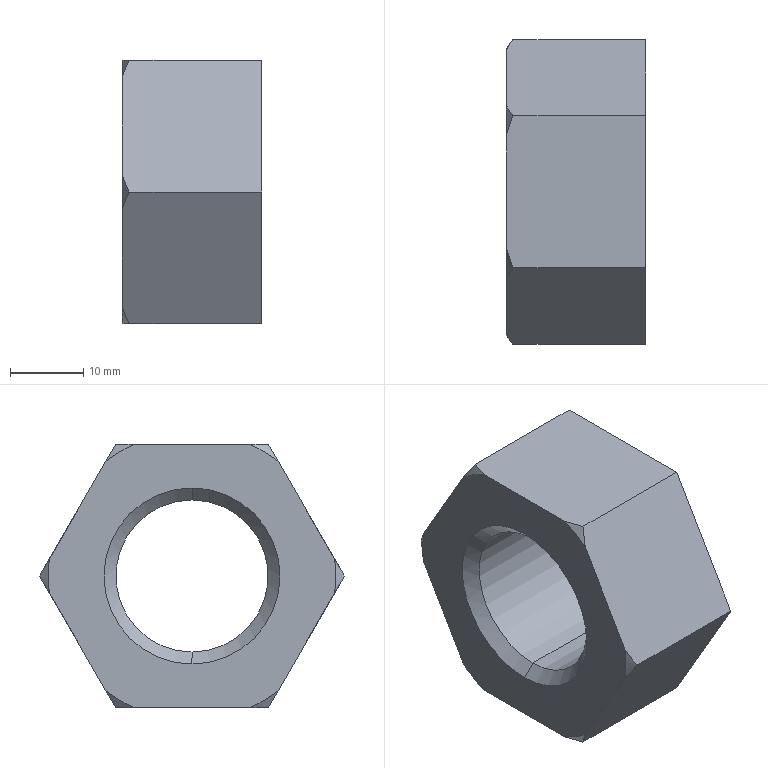Part | STEP file | 11-FJFN24nut11 | 1 solid | 20 faces | box 19 x 41.569 x 36 mm | volume 14713 mm3 | cone 10 | plane 8 | cylinder 2 | commonest cylinder face diameters 20.752 x2
STEP:
#1=CARTESIAN_POINT('',(17.376,0.,-10.376));
#2=VERTEX_POINT('',#1);
#3=CARTESIAN_POINT('',(17.376,0.,10.376));
#4=VERTEX_POINT('',#3);
#5=CARTESIAN_POINT('',(17.376,0.,0.));
#6=DIRECTION('',(-1.,0.,0.));
#7=DIRECTION('',(0.,0.,1.));
#8=AXIS2_PLACEMENT_3D('',#5,#6,#7);
#9=CIRCLE('',#8,10.376);
#10=EDGE_CURVE('',#2,#4,#9,.T.);
#11=ORIENTED_EDGE('',*,*,#10,.T.);
#12=CARTESIAN_POINT('',(19.,0.,12.));
#13=VERTEX_POINT('',#12);
#14=CARTESIAN_POINT('',(17.376,0.,10.376));
#15=DIRECTION('',(0.7071,0.,0.7071));
#16=VECTOR('',#15,1000.);
#17=LINE('',#14,#16);
#18=EDGE_CURVE('',#4,#13,#17,.T.);
#19=ORIENTED_EDGE('',*,*,#18,.T.);
#20=CARTESIAN_POINT('',(19.,0.,-12.));
#21=VERTEX_POINT('',#20);
#22=CARTESIAN_POINT('',(19.,0.,0.));
#23=DIRECTION('',(-1.,0.,0.));
#24=DIRECTION('',(0.,0.,1.));
#25=AXIS2_PLACEMENT_3D('',#22,#23,#24);
#26=CIRCLE('',#25,12.);
#27=EDGE_CURVE('',#21,#13,#26,.T.);
#28=ORIENTED_EDGE('',*,*,#27,.F.);
#29=CARTESIAN_POINT('',(17.376,0.,-10.376));
#30=DIRECTION('',(0.7071,0.,-0.7071));
#31=VECTOR('',#30,1000.);
#32=LINE('',#29,#31);
#33=EDGE_CURVE('',#2,#21,#32,.T.);
#34=ORIENTED_EDGE('',*,*,#33,.F.);
#35=EDGE_LOOP('',(#11,#19,#28,#34));
#36=FACE_OUTER_BOUND('',#35,.T.);
#37=CARTESIAN_POINT('',(17.376,0.,0.));
#38=DIRECTION('',(1.,0.,0.));
#39=DIRECTION('',(0.,0.,-1.));
#40=AXIS2_PLACEMENT_3D('',#37,#38,#39);
#41=CONICAL_SURFACE('',#40,10.376,0.7854);
#42=ADVANCED_FACE('',(#36),#41,.F.);
#43=ORIENTED_EDGE('',*,*,#10,.F.);
#44=CARTESIAN_POINT('',(1.624,0.,-10.376));
#45=VERTEX_POINT('',#44);
#46=CARTESIAN_POINT('',(19.,0.,-10.376));
#47=DIRECTION('',(-1.,0.,0.));
#48=VECTOR('',#47,1000.);
#49=LINE('',#46,#48);
#50=EDGE_CURVE('',#2,#45,#49,.T.);
#51=ORIENTED_EDGE('',*,*,#50,.T.);
#52=CARTESIAN_POINT('',(1.624,0.,10.376));
#53=VERTEX_POINT('',#52);
#54=CARTESIAN_POINT('',(1.624,0.,0.));
#55=DIRECTION('',(-1.,0.,0.));
#56=DIRECTION('',(0.,0.,1.));
#57=AXIS2_PLACEMENT_3D('',#54,#55,#56);
#58=CIRCLE('',#57,10.376);
#59=EDGE_CURVE('',#45,#53,#58,.T.);
#60=ORIENTED_EDGE('',*,*,#59,.T.);
#61=CARTESIAN_POINT('',(19.,0.,10.376));
#62=DIRECTION('',(-1.,0.,0.));
#63=VECTOR('',#62,1000.);
#64=LINE('',#61,#63);
#65=EDGE_CURVE('',#4,#53,#64,.T.);
#66=ORIENTED_EDGE('',*,*,#65,.F.);
#67=EDGE_LOOP('',(#43,#51,#60,#66));
#68=FACE_OUTER_BOUND('',#67,.T.);
#69=CARTESIAN_POINT('',(19.,0.,0.));
#70=DIRECTION('',(-1.,0.,0.));
#71=DIRECTION('',(0.,0.,1.));
#72=AXIS2_PLACEMENT_3D('',#69,#70,#71);
#73=CYLINDRICAL_SURFACE('',#72,10.376);
#74=ADVANCED_FACE('',(#68),#73,.F.);
#75=ORIENTED_EDGE('',*,*,#59,.F.);
#76=CARTESIAN_POINT('',(0.,0.,-12.));
#77=VERTEX_POINT('',#76);
#78=CARTESIAN_POINT('',(0.,0.,-12.));
#79=DIRECTION('',(-0.7071,0.,-0.7071));
#80=VECTOR('',#79,1000.);
#81=LINE('',#78,#80);
#82=EDGE_CURVE('',#45,#77,#81,.T.);
#83=ORIENTED_EDGE('',*,*,#82,.T.);
#84=CARTESIAN_POINT('',(0.,0.,12.));
#85=VERTEX_POINT('',#84);
#86=CARTESIAN_POINT('',(0.,0.,0.));
#87=DIRECTION('',(-1.,0.,0.));
#88=DIRECTION('',(0.,0.,1.));
#89=AXIS2_PLACEMENT_3D('',#86,#87,#88);
#90=CIRCLE('',#89,12.);
#91=EDGE_CURVE('',#77,#85,#90,.T.);
#92=ORIENTED_EDGE('',*,*,#91,.T.);
#93=CARTESIAN_POINT('',(0.,0.,12.));
#94=DIRECTION('',(-0.7071,0.,0.7071));
#95=VECTOR('',#94,1000.);
#96=LINE('',#93,#95);
#97=EDGE_CURVE('',#53,#85,#96,.T.);
#98=ORIENTED_EDGE('',*,*,#97,.F.);
#99=EDGE_LOOP('',(#75,#83,#92,#98));
#100=FACE_OUTER_BOUND('',#99,.T.);
#101=CARTESIAN_POINT('',(0.,0.,0.));
#102=DIRECTION('',(-1.,0.,0.));
#103=DIRECTION('',(0.,0.,1.));
#104=AXIS2_PLACEMENT_3D('',#101,#102,#103);
#105=CONICAL_SURFACE('',#104,12.,0.7854);
#106=ADVANCED_FACE('',(#100),#105,.F.);
#107=CARTESIAN_POINT('',(0.,7.756,18.));
#108=VERTEX_POINT('',#107);
#109=CARTESIAN_POINT('',(0.8885,10.392,18.));
#110=VERTEX_POINT('',#109);
#111=CARTESIAN_POINT('',(0.,7.756,18.));
#112=CARTESIAN_POINT('',(0.2629,8.642,18.));
#113=CARTESIAN_POINT('',(0.5623,9.523,18.));
#114=CARTESIAN_POINT('',(0.8885,10.392,18.));
#115=B_SPLINE_CURVE_WITH_KNOTS('',3,(#111,#112,#113,#114),.UNSPECIFIED.,.F.,.F.,(4,4),(0.03246,0.03523),.UNSPECIFIED.);
#116=EDGE_CURVE('',#108,#110,#115,.T.);
#117=ORIENTED_EDGE('',*,*,#116,.T.);
#118=CARTESIAN_POINT('',(0.,11.71,15.717));
#119=VERTEX_POINT('',#118);
#120=CARTESIAN_POINT('',(0.8885,10.392,18.));
#121=CARTESIAN_POINT('',(0.5616,10.828,17.245));
#122=CARTESIAN_POINT('',(0.2631,11.267,16.485));
#123=CARTESIAN_POINT('',(0.,11.71,15.717));
#124=B_SPLINE_CURVE_WITH_KNOTS('',3,(#120,#121,#122,#123),.UNSPECIFIED.,.F.,.F.,(4,4),(0.01623,0.01901),.UNSPECIFIED.);
#125=EDGE_CURVE('',#110,#119,#124,.T.);
#126=ORIENTED_EDGE('',*,*,#125,.T.);
#127=CARTESIAN_POINT('',(0.,0.,0.));
#128=DIRECTION('',(-1.,0.,0.));
#129=DIRECTION('',(0.,0.,1.));
#130=AXIS2_PLACEMENT_3D('',#127,#128,#129);
#131=CIRCLE('',#130,19.6);
#132=EDGE_CURVE('',#108,#119,#131,.T.);
#133=ORIENTED_EDGE('',*,*,#132,.F.);
#134=EDGE_LOOP('',(#117,#126,#133));
#135=FACE_OUTER_BOUND('',#134,.T.);
#136=CARTESIAN_POINT('',(1.5,0.,0.));
#137=DIRECTION('',(1.,0.,0.));
#138=DIRECTION('',(0.,0.,-1.));
#139=AXIS2_PLACEMENT_3D('',#136,#137,#138);
#140=CONICAL_SURFACE('',#139,21.6,0.9273);
#141=ADVANCED_FACE('',(#135),#140,.T.);
#142=CARTESIAN_POINT('',(0.,-11.71,15.717));
#143=VERTEX_POINT('',#142);
#144=CARTESIAN_POINT('',(0.8885,-10.392,18.));
#145=VERTEX_POINT('',#144);
#146=CARTESIAN_POINT('',(0.,-11.71,15.717));
#147=CARTESIAN_POINT('',(0.2644,-11.265,16.489));
#148=CARTESIAN_POINT('',(0.564,-10.825,17.251));
#149=CARTESIAN_POINT('',(0.8885,-10.392,18.));
#150=B_SPLINE_CURVE_WITH_KNOTS('',3,(#146,#147,#148,#149),.UNSPECIFIED.,.F.,.F.,(4,4),(0.03478,0.03755),.UNSPECIFIED.);
#151=EDGE_CURVE('',#143,#145,#150,.T.);
#152=ORIENTED_EDGE('',*,*,#151,.T.);
#153=CARTESIAN_POINT('',(0.,-7.756,18.));
#154=VERTEX_POINT('',#153);
#155=CARTESIAN_POINT('',(0.8885,-10.392,18.));
#156=CARTESIAN_POINT('',(0.5638,-9.526,18.));
#157=CARTESIAN_POINT('',(0.2638,-8.645,18.));
#158=CARTESIAN_POINT('',(0.,-7.756,18.));
#159=B_SPLINE_CURVE_WITH_KNOTS('',3,(#155,#156,#157,#158),.UNSPECIFIED.,.F.,.F.,(4,4),(0.01398,0.01674),.UNSPECIFIED.);
#160=EDGE_CURVE('',#145,#154,#159,.T.);
#161=ORIENTED_EDGE('',*,*,#160,.T.);
#162=CARTESIAN_POINT('',(0.,0.,0.));
#163=DIRECTION('',(-1.,0.,0.));
#164=DIRECTION('',(0.,0.,1.));
#165=AXIS2_PLACEMENT_3D('',#162,#163,#164);
#166=CIRCLE('',#165,19.6);
#167=EDGE_CURVE('',#143,#154,#166,.T.);
#168=ORIENTED_EDGE('',*,*,#167,.F.);
#169=EDGE_LOOP('',(#152,#161,#168));
#170=FACE_OUTER_BOUND('',#169,.T.);
#171=CARTESIAN_POINT('',(1.5,0.,0.));
#172=DIRECTION('',(1.,0.,0.));
#173=DIRECTION('',(0.,0.,-1.));
#174=AXIS2_PLACEMENT_3D('',#171,#172,#173);
#175=CONICAL_SURFACE('',#174,21.6,0.9273);
#176=ADVANCED_FACE('',(#170),#175,.T.);
#177=CARTESIAN_POINT('',(0.,-19.467,-2.283));
#178=VERTEX_POINT('',#177);
#179=CARTESIAN_POINT('',(0.8885,-20.785,0.));
#180=VERTEX_POINT('',#179);
#181=CARTESIAN_POINT('',(0.,-19.467,-2.283));
#182=CARTESIAN_POINT('',(0.2644,-19.912,-1.511));
#183=CARTESIAN_POINT('',(0.564,-20.352,-0.7492));
#184=CARTESIAN_POINT('',(0.8885,-20.785,0.));
#185=B_SPLINE_CURVE_WITH_KNOTS('',3,(#181,#182,#183,#184),.UNSPECIFIED.,.F.,.F.,(4,4),(0.03478,0.03755),.UNSPECIFIED.);
#186=EDGE_CURVE('',#178,#180,#185,.T.);
#187=ORIENTED_EDGE('',*,*,#186,.T.);
#188=CARTESIAN_POINT('',(0.,-19.467,2.283));
#189=VERTEX_POINT('',#188);
#190=CARTESIAN_POINT('',(0.8885,-20.785,0.));
#191=CARTESIAN_POINT('',(0.5616,-20.349,0.7548));
#192=CARTESIAN_POINT('',(0.2631,-19.91,1.515));
#193=CARTESIAN_POINT('',(0.,-19.467,2.283));
#194=B_SPLINE_CURVE_WITH_KNOTS('',3,(#190,#191,#192,#193),.UNSPECIFIED.,.F.,.F.,(4,4),(0.01623,0.01901),.UNSPECIFIED.);
#195=EDGE_CURVE('',#180,#189,#194,.T.);
#196=ORIENTED_EDGE('',*,*,#195,.T.);
#197=CARTESIAN_POINT('',(0.,0.,0.));
#198=DIRECTION('',(-1.,0.,0.));
#199=DIRECTION('',(0.,0.,1.));
#200=AXIS2_PLACEMENT_3D('',#197,#198,#199);
#201=CIRCLE('',#200,19.6);
#202=EDGE_CURVE('',#178,#189,#201,.T.);
#203=ORIENTED_EDGE('',*,*,#202,.F.);
#204=EDGE_LOOP('',(#187,#196,#203));
#205=FACE_OUTER_BOUND('',#204,.T.);
#206=CARTESIAN_POINT('',(1.5,0.,0.));
#207=DIRECTION('',(1.,0.,0.));
#208=DIRECTION('',(0.,0.,-1.));
#209=AXIS2_PLACEMENT_3D('',#206,#207,#208);
#210=CONICAL_SURFACE('',#209,21.6,0.9273);
#211=ADVANCED_FACE('',(#205),#210,.T.);
#212=CARTESIAN_POINT('',(0.,-7.756,-18.));
#213=VERTEX_POINT('',#212);
#214=CARTESIAN_POINT('',(0.8885,-10.392,-18.));
#215=VERTEX_POINT('',#214);
#216=CARTESIAN_POINT('',(0.,-7.756,-18.));
#217=CARTESIAN_POINT('',(0.2629,-8.642,-18.));
#218=CARTESIAN_POINT('',(0.5623,-9.523,-18.));
#219=CARTESIAN_POINT('',(0.8885,-10.392,-18.));
#220=B_SPLINE_CURVE_WITH_KNOTS('',3,(#216,#217,#218,#219),.UNSPECIFIED.,.F.,.F.,(4,4),(0.03246,0.03523),.UNSPECIFIED.);
#221=EDGE_CURVE('',#213,#215,#220,.T.);
#222=ORIENTED_EDGE('',*,*,#221,.T.);
#223=CARTESIAN_POINT('',(0.,-11.71,-15.717));
#224=VERTEX_POINT('',#223);
#225=CARTESIAN_POINT('',(0.8885,-10.392,-18.));
#226=CARTESIAN_POINT('',(0.5616,-10.828,-17.245));
#227=CARTESIAN_POINT('',(0.2631,-11.267,-16.485));
#228=CARTESIAN_POINT('',(0.,-11.71,-15.717));
#229=B_SPLINE_CURVE_WITH_KNOTS('',3,(#225,#226,#227,#228),.UNSPECIFIED.,.F.,.F.,(4,4),(0.01623,0.01901),.UNSPECIFIED.);
#230=EDGE_CURVE('',#215,#224,#229,.T.);
#231=ORIENTED_EDGE('',*,*,#230,.T.);
#232=CARTESIAN_POINT('',(0.,0.,0.));
#233=DIRECTION('',(-1.,0.,0.));
#234=DIRECTION('',(0.,0.,1.));
#235=AXIS2_PLACEMENT_3D('',#232,#233,#234);
#236=CIRCLE('',#235,19.6);
#237=EDGE_CURVE('',#213,#224,#236,.T.);
#238=ORIENTED_EDGE('',*,*,#237,.F.);
#239=EDGE_LOOP('',(#222,#231,#238));
#240=FACE_OUTER_BOUND('',#239,.T.);
#241=CARTESIAN_POINT('',(1.5,0.,0.));
#242=DIRECTION('',(1.,0.,0.));
#243=DIRECTION('',(0.,0.,-1.));
#244=AXIS2_PLACEMENT_3D('',#241,#242,#243);
#245=CONICAL_SURFACE('',#244,21.6,0.9273);
#246=ADVANCED_FACE('',(#240),#245,.T.);
#247=CARTESIAN_POINT('',(0.,19.467,2.283));
#248=VERTEX_POINT('',#247);
#249=CARTESIAN_POINT('',(0.,19.467,-2.283));
#250=VERTEX_POINT('',#249);
#251=CARTESIAN_POINT('',(0.,0.,0.));
#252=DIRECTION('',(-1.,0.,0.));
#253=DIRECTION('',(0.,0.,1.));
#254=AXIS2_PLACEMENT_3D('',#251,#252,#253);
#255=CIRCLE('',#254,19.6);
#256=EDGE_CURVE('',#248,#250,#255,.T.);
#257=ORIENTED_EDGE('',*,*,#256,.F.);
#258=CARTESIAN_POINT('',(0.8885,20.785,0.));
#259=VERTEX_POINT('',#258);
#260=CARTESIAN_POINT('',(0.,19.467,2.283));
#261=CARTESIAN_POINT('',(0.2644,19.912,1.511));
#262=CARTESIAN_POINT('',(0.564,20.352,0.7492));
#263=CARTESIAN_POINT('',(0.8885,20.785,0.));
#264=B_SPLINE_CURVE_WITH_KNOTS('',3,(#260,#261,#262,#263),.UNSPECIFIED.,.F.,.F.,(4,4),(0.03478,0.03755),.UNSPECIFIED.);
#265=EDGE_CURVE('',#248,#259,#264,.T.);
#266=ORIENTED_EDGE('',*,*,#265,.T.);
#267=CARTESIAN_POINT('',(0.8885,20.785,0.));
#268=CARTESIAN_POINT('',(0.5616,20.349,-0.7548));
#269=CARTESIAN_POINT('',(0.2631,19.91,-1.515));
#270=CARTESIAN_POINT('',(0.,19.467,-2.283));
#271=B_SPLINE_CURVE_WITH_KNOTS('',3,(#267,#268,#269,#270),.UNSPECIFIED.,.F.,.F.,(4,4),(0.01623,0.01901),.UNSPECIFIED.);
#272=EDGE_CURVE('',#259,#250,#271,.T.);
#273=ORIENTED_EDGE('',*,*,#272,.T.);
#274=EDGE_LOOP('',(#257,#266,#273));
#275=FACE_OUTER_BOUND('',#274,.T.);
#276=CARTESIAN_POINT('',(1.5,0.,0.));
#277=DIRECTION('',(1.,0.,0.));
#278=DIRECTION('',(0.,0.,-1.));
#279=AXIS2_PLACEMENT_3D('',#276,#277,#278);
#280=CONICAL_SURFACE('',#279,21.6,0.9273);
#281=ADVANCED_FACE('',(#275),#280,.T.);
#282=CARTESIAN_POINT('',(0.,11.71,-15.717));
#283=VERTEX_POINT('',#282);
#284=CARTESIAN_POINT('',(0.8885,10.392,-18.));
#285=VERTEX_POINT('',#284);
#286=CARTESIAN_POINT('',(0.,11.71,-15.717));
#287=CARTESIAN_POINT('',(0.2644,11.265,-16.489));
#288=CARTESIAN_POINT('',(0.564,10.825,-17.251));
#289=CARTESIAN_POINT('',(0.8885,10.392,-18.));
#290=B_SPLINE_CURVE_WITH_KNOTS('',3,(#286,#287,#288,#289),.UNSPECIFIED.,.F.,.F.,(4,4),(0.03478,0.03755),.UNSPECIFIED.);
#291=EDGE_CURVE('',#283,#285,#290,.T.);
#292=ORIENTED_EDGE('',*,*,#291,.T.);
#293=CARTESIAN_POINT('',(0.,7.756,-18.));
#294=VERTEX_POINT('',#293);
#295=CARTESIAN_POINT('',(0.8885,10.392,-18.));
#296=CARTESIAN_POINT('',(0.5638,9.526,-18.));
#297=CARTESIAN_POINT('',(0.2638,8.645,-18.));
#298=CARTESIAN_POINT('',(0.,7.756,-18.));
#299=B_SPLINE_CURVE_WITH_KNOTS('',3,(#295,#296,#297,#298),.UNSPECIFIED.,.F.,.F.,(4,4),(0.01398,0.01674),.UNSPECIFIED.);
#300=EDGE_CURVE('',#285,#294,#299,.T.);
#301=ORIENTED_EDGE('',*,*,#300,.T.);
#302=CARTESIAN_POINT('',(0.,0.,0.));
#303=DIRECTION('',(-1.,0.,0.));
#304=DIRECTION('',(0.,0.,1.));
#305=AXIS2_PLACEMENT_3D('',#302,#303,#304);
#306=CIRCLE('',#305,19.6);
#307=EDGE_CURVE('',#283,#294,#306,.T.);
#308=ORIENTED_EDGE('',*,*,#307,.F.);
#309=EDGE_LOOP('',(#292,#301,#308));
#310=FACE_OUTER_BOUND('',#309,.T.);
#311=CARTESIAN_POINT('',(1.5,0.,0.));
#312=DIRECTION('',(1.,0.,0.));
#313=DIRECTION('',(0.,0.,-1.));
#314=AXIS2_PLACEMENT_3D('',#311,#312,#313);
#315=CONICAL_SURFACE('',#314,21.6,0.9273);
#316=ADVANCED_FACE('',(#310),#315,.T.);
#317=CARTESIAN_POINT('',(0.,0.,0.));
#318=DIRECTION('',(-1.,0.,0.));
#319=DIRECTION('',(0.,0.,1.));
#320=AXIS2_PLACEMENT_3D('',#317,#318,#319);
#321=CIRCLE('',#320,12.);
#322=EDGE_CURVE('',#85,#77,#321,.T.);
#323=ORIENTED_EDGE('',*,*,#322,.F.);
#324=ORIENTED_EDGE('',*,*,#91,.F.);
#325=EDGE_LOOP('',(#323,#324));
#326=FACE_BOUND('',#325,.T.);
#327=ORIENTED_EDGE('',*,*,#132,.T.);
#328=CARTESIAN_POINT('',(0.,20.785,0.));
#329=DIRECTION('',(0.,-0.5,0.866));
#330=VECTOR('',#329,1000.);
#331=LINE('',#328,#330);
#332=EDGE_CURVE('',#248,#119,#331,.T.);
#333=ORIENTED_EDGE('',*,*,#332,.F.);
#334=ORIENTED_EDGE('',*,*,#256,.T.);
#335=CARTESIAN_POINT('',(0.,10.392,-18.));
#336=DIRECTION('',(0.,0.5,0.866));
#337=VECTOR('',#336,1000.);
#338=LINE('',#335,#337);
#339=EDGE_CURVE('',#283,#250,#338,.T.);
#340=ORIENTED_EDGE('',*,*,#339,.F.);
#341=ORIENTED_EDGE('',*,*,#307,.T.);
#342=CARTESIAN_POINT('',(0.,-10.392,-18.));
#343=DIRECTION('',(0.,1.,0.));
#344=VECTOR('',#343,1000.);
#345=LINE('',#342,#344);
#346=EDGE_CURVE('',#213,#294,#345,.T.);
#347=ORIENTED_EDGE('',*,*,#346,.F.);
#348=ORIENTED_EDGE('',*,*,#237,.T.);
#349=CARTESIAN_POINT('',(0.,-20.785,0.));
#350=DIRECTION('',(0.,0.5,-0.866));
#351=VECTOR('',#350,1000.);
#352=LINE('',#349,#351);
#353=EDGE_CURVE('',#178,#224,#352,.T.);
#354=ORIENTED_EDGE('',*,*,#353,.F.);
#355=ORIENTED_EDGE('',*,*,#202,.T.);
#356=CARTESIAN_POINT('',(0.,-10.392,18.));
#357=DIRECTION('',(0.,-0.5,-0.866));
#358=VECTOR('',#357,1000.);
#359=LINE('',#356,#358);
#360=EDGE_CURVE('',#143,#189,#359,.T.);
#361=ORIENTED_EDGE('',*,*,#360,.F.);
#362=ORIENTED_EDGE('',*,*,#167,.T.);
#363=CARTESIAN_POINT('',(0.,10.392,18.));
#364=DIRECTION('',(0.,-1.,0.));
#365=VECTOR('',#364,1000.);
#366=LINE('',#363,#365);
#367=EDGE_CURVE('',#108,#154,#366,.T.);
#368=ORIENTED_EDGE('',*,*,#367,.F.);
#369=EDGE_LOOP('',(#327,#333,#334,#340,#341,#347,#348,#354,#355,#361,#362,#368));
#370=FACE_OUTER_BOUND('',#369,.T.);
#371=CARTESIAN_POINT('',(0.,19.6,0.));
#372=DIRECTION('',(1.,0.,0.));
#373=DIRECTION('',(0.,0.,-1.));
#374=AXIS2_PLACEMENT_3D('',#371,#372,#373);
#375=PLANE('',#374);
#376=ADVANCED_FACE('',(#326,#370),#375,.F.);
#377=ORIENTED_EDGE('',*,*,#82,.F.);
#378=CARTESIAN_POINT('',(1.624,0.,0.));
#379=DIRECTION('',(-1.,0.,0.));
#380=DIRECTION('',(0.,0.,1.));
#381=AXIS2_PLACEMENT_3D('',#378,#379,#380);
#382=CIRCLE('',#381,10.376);
#383=EDGE_CURVE('',#53,#45,#382,.T.);
#384=ORIENTED_EDGE('',*,*,#383,.F.);
#385=ORIENTED_EDGE('',*,*,#97,.T.);
#386=ORIENTED_EDGE('',*,*,#322,.T.);
#387=EDGE_LOOP('',(#377,#384,#385,#386));
#388=FACE_OUTER_BOUND('',#387,.T.);
#389=CARTESIAN_POINT('',(0.,0.,0.));
#390=DIRECTION('',(-1.,0.,0.));
#391=DIRECTION('',(0.,0.,1.));
#392=AXIS2_PLACEMENT_3D('',#389,#390,#391);
#393=CONICAL_SURFACE('',#392,12.,0.7854);
#394=ADVANCED_FACE('',(#388),#393,.F.);
#395=ORIENTED_EDGE('',*,*,#50,.F.);
#396=CARTESIAN_POINT('',(17.376,0.,0.));
#397=DIRECTION('',(-1.,0.,0.));
#398=DIRECTION('',(0.,0.,1.));
#399=AXIS2_PLACEMENT_3D('',#396,#397,#398);
#400=CIRCLE('',#399,10.376);
#401=EDGE_CURVE('',#4,#2,#400,.T.);
#402=ORIENTED_EDGE('',*,*,#401,.F.);
#403=ORIENTED_EDGE('',*,*,#65,.T.);
#404=ORIENTED_EDGE('',*,*,#383,.T.);
#405=EDGE_LOOP('',(#395,#402,#403,#404));
#406=FACE_OUTER_BOUND('',#405,.T.);
#407=CARTESIAN_POINT('',(19.,0.,0.));
#408=DIRECTION('',(-1.,0.,0.));
#409=DIRECTION('',(0.,0.,1.));
#410=AXIS2_PLACEMENT_3D('',#407,#408,#409);
#411=CYLINDRICAL_SURFACE('',#410,10.376);
#412=ADVANCED_FACE('',(#406),#411,.F.);
#413=ORIENTED_EDGE('',*,*,#18,.F.);
#414=ORIENTED_EDGE('',*,*,#401,.T.);
#415=ORIENTED_EDGE('',*,*,#33,.T.);
#416=CARTESIAN_POINT('',(19.,0.,0.));
#417=DIRECTION('',(-1.,0.,0.));
#418=DIRECTION('',(0.,0.,1.));
#419=AXIS2_PLACEMENT_3D('',#416,#417,#418);
#420=CIRCLE('',#419,12.);
#421=EDGE_CURVE('',#13,#21,#420,.T.);
#422=ORIENTED_EDGE('',*,*,#421,.F.);
#423=EDGE_LOOP('',(#413,#414,#415,#422));
#424=FACE_OUTER_BOUND('',#423,.T.);
#425=CARTESIAN_POINT('',(17.376,0.,0.));
#426=DIRECTION('',(1.,0.,0.));
#427=DIRECTION('',(0.,0.,-1.));
#428=AXIS2_PLACEMENT_3D('',#425,#426,#427);
#429=CONICAL_SURFACE('',#428,10.376,0.7854);
#430=ADVANCED_FACE('',(#424),#429,.F.);
#431=CARTESIAN_POINT('',(19.,10.392,-18.));
#432=VERTEX_POINT('',#431);
#433=CARTESIAN_POINT('',(19.,20.785,0.));
#434=VERTEX_POINT('',#433);
#435=CARTESIAN_POINT('',(19.,10.392,-18.));
#436=DIRECTION('',(0.,0.5,0.866));
#437=VECTOR('',#436,1000.);
#438=LINE('',#435,#437);
#439=EDGE_CURVE('',#432,#434,#438,.T.);
#440=ORIENTED_EDGE('',*,*,#439,.T.);
#441=CARTESIAN_POINT('',(19.,10.392,18.));
#442=VERTEX_POINT('',#441);
#443=CARTESIAN_POINT('',(19.,20.785,0.));
#444=DIRECTION('',(0.,-0.5,0.866));
#445=VECTOR('',#444,1000.);
#446=LINE('',#443,#445);
#447=EDGE_CURVE('',#434,#442,#446,.T.);
#448=ORIENTED_EDGE('',*,*,#447,.T.);
#449=CARTESIAN_POINT('',(19.,-10.392,18.));
#450=VERTEX_POINT('',#449);
#451=CARTESIAN_POINT('',(19.,10.392,18.));
#452=DIRECTION('',(0.,-1.,0.));
#453=VECTOR('',#452,1000.);
#454=LINE('',#451,#453);
#455=EDGE_CURVE('',#442,#450,#454,.T.);
#456=ORIENTED_EDGE('',*,*,#455,.T.);
#457=CARTESIAN_POINT('',(19.,-20.785,0.));
#458=VERTEX_POINT('',#457);
#459=CARTESIAN_POINT('',(19.,-10.392,18.));
#460=DIRECTION('',(0.,-0.5,-0.866));
#461=VECTOR('',#460,1000.);
#462=LINE('',#459,#461);
#463=EDGE_CURVE('',#450,#458,#462,.T.);
#464=ORIENTED_EDGE('',*,*,#463,.T.);
#465=CARTESIAN_POINT('',(19.,-10.392,-18.));
#466=VERTEX_POINT('',#465);
#467=CARTESIAN_POINT('',(19.,-20.785,0.));
#468=DIRECTION('',(0.,0.5,-0.866));
#469=VECTOR('',#468,1000.);
#470=LINE('',#467,#469);
#471=EDGE_CURVE('',#458,#466,#470,.T.);
#472=ORIENTED_EDGE('',*,*,#471,.T.);
#473=CARTESIAN_POINT('',(19.,-10.392,-18.));
#474=DIRECTION('',(0.,1.,0.));
#475=VECTOR('',#474,1000.);
#476=LINE('',#473,#475);
#477=EDGE_CURVE('',#466,#432,#476,.T.);
#478=ORIENTED_EDGE('',*,*,#477,.T.);
#479=EDGE_LOOP('',(#440,#448,#456,#464,#472,#478));
#480=FACE_OUTER_BOUND('',#479,.T.);
#481=ORIENTED_EDGE('',*,*,#27,.T.);
#482=ORIENTED_EDGE('',*,*,#421,.T.);
#483=EDGE_LOOP('',(#481,#482));
#484=FACE_BOUND('',#483,.T.);
#485=CARTESIAN_POINT('',(19.,12.,0.));
#486=DIRECTION('',(-1.,0.,0.));
#487=DIRECTION('',(0.,0.,1.));
#488=AXIS2_PLACEMENT_3D('',#485,#486,#487);
#489=PLANE('',#488);
#490=ADVANCED_FACE('',(#480,#484),#489,.F.);
#491=CARTESIAN_POINT('',(19.,10.392,18.));
#492=DIRECTION('',(-1.,0.,0.));
#493=VECTOR('',#492,1000.);
#494=LINE('',#491,#493);
#495=EDGE_CURVE('',#442,#110,#494,.T.);
#496=ORIENTED_EDGE('',*,*,#495,.F.);
#497=ORIENTED_EDGE('',*,*,#447,.F.);
#498=CARTESIAN_POINT('',(19.,20.785,0.));
#499=DIRECTION('',(-1.,0.,0.));
#500=VECTOR('',#499,1000.);
#501=LINE('',#498,#500);
#502=EDGE_CURVE('',#434,#259,#501,.T.);
#503=ORIENTED_EDGE('',*,*,#502,.T.);
#504=ORIENTED_EDGE('',*,*,#265,.F.);
#505=ORIENTED_EDGE('',*,*,#332,.T.);
#506=ORIENTED_EDGE('',*,*,#125,.F.);
#507=EDGE_LOOP('',(#496,#497,#503,#504,#505,#506));
#508=FACE_OUTER_BOUND('',#507,.T.);
#509=CARTESIAN_POINT('',(19.,20.785,0.));
#510=DIRECTION('',(0.,-0.866,-0.5));
#511=DIRECTION('',(0.,0.5,-0.866));
#512=AXIS2_PLACEMENT_3D('',#509,#510,#511);
#513=PLANE('',#512);
#514=ADVANCED_FACE('',(#508),#513,.F.);
#515=CARTESIAN_POINT('',(19.,-10.392,18.));
#516=DIRECTION('',(-1.,0.,0.));
#517=VECTOR('',#516,1000.);
#518=LINE('',#515,#517);
#519=EDGE_CURVE('',#450,#145,#518,.T.);
#520=ORIENTED_EDGE('',*,*,#519,.F.);
#521=ORIENTED_EDGE('',*,*,#455,.F.);
#522=ORIENTED_EDGE('',*,*,#495,.T.);
#523=ORIENTED_EDGE('',*,*,#116,.F.);
#524=ORIENTED_EDGE('',*,*,#367,.T.);
#525=ORIENTED_EDGE('',*,*,#160,.F.);
#526=EDGE_LOOP('',(#520,#521,#522,#523,#524,#525));
#527=FACE_OUTER_BOUND('',#526,.T.);
#528=CARTESIAN_POINT('',(19.,10.392,18.));
#529=DIRECTION('',(0.,0.,-1.));
#530=DIRECTION('',(-1.,0.,0.));
#531=AXIS2_PLACEMENT_3D('',#528,#529,#530);
#532=PLANE('',#531);
#533=ADVANCED_FACE('',(#527),#532,.F.);
#534=CARTESIAN_POINT('',(19.,-20.785,0.));
#535=DIRECTION('',(-1.,0.,0.));
#536=VECTOR('',#535,1000.);
#537=LINE('',#534,#536);
#538=EDGE_CURVE('',#458,#180,#537,.T.);
#539=ORIENTED_EDGE('',*,*,#538,.F.);
#540=ORIENTED_EDGE('',*,*,#463,.F.);
#541=ORIENTED_EDGE('',*,*,#519,.T.);
#542=ORIENTED_EDGE('',*,*,#151,.F.);
#543=ORIENTED_EDGE('',*,*,#360,.T.);
#544=ORIENTED_EDGE('',*,*,#195,.F.);
#545=EDGE_LOOP('',(#539,#540,#541,#542,#543,#544));
#546=FACE_OUTER_BOUND('',#545,.T.);
#547=CARTESIAN_POINT('',(19.,-10.392,18.));
#548=DIRECTION('',(0.,0.866,-0.5));
#549=DIRECTION('',(0.,0.5,0.866));
#550=AXIS2_PLACEMENT_3D('',#547,#548,#549);
#551=PLANE('',#550);
#552=ADVANCED_FACE('',(#546),#551,.F.);
#553=CARTESIAN_POINT('',(19.,-10.392,-18.));
#554=DIRECTION('',(-1.,0.,0.));
#555=VECTOR('',#554,1000.);
#556=LINE('',#553,#555);
#557=EDGE_CURVE('',#466,#215,#556,.T.);
#558=ORIENTED_EDGE('',*,*,#557,.F.);
#559=ORIENTED_EDGE('',*,*,#471,.F.);
#560=ORIENTED_EDGE('',*,*,#538,.T.);
#561=ORIENTED_EDGE('',*,*,#186,.F.);
#562=ORIENTED_EDGE('',*,*,#353,.T.);
#563=ORIENTED_EDGE('',*,*,#230,.F.);
#564=EDGE_LOOP('',(#558,#559,#560,#561,#562,#563));
#565=FACE_OUTER_BOUND('',#564,.T.);
#566=CARTESIAN_POINT('',(19.,-20.785,0.));
#567=DIRECTION('',(0.,0.866,0.5));
#568=DIRECTION('',(0.,-0.5,0.866));
#569=AXIS2_PLACEMENT_3D('',#566,#567,#568);
#570=PLANE('',#569);
#571=ADVANCED_FACE('',(#565),#570,.F.);
#572=CARTESIAN_POINT('',(19.,10.392,-18.));
#573=DIRECTION('',(-1.,0.,0.));
#574=VECTOR('',#573,1000.);
#575=LINE('',#572,#574);
#576=EDGE_CURVE('',#432,#285,#575,.T.);
#577=ORIENTED_EDGE('',*,*,#576,.F.);
#578=ORIENTED_EDGE('',*,*,#477,.F.);
#579=ORIENTED_EDGE('',*,*,#557,.T.);
#580=ORIENTED_EDGE('',*,*,#221,.F.);
#581=ORIENTED_EDGE('',*,*,#346,.T.);
#582=ORIENTED_EDGE('',*,*,#300,.F.);
#583=EDGE_LOOP('',(#577,#578,#579,#580,#581,#582));
#584=FACE_OUTER_BOUND('',#583,.T.);
#585=CARTESIAN_POINT('',(19.,-10.392,-18.));
#586=DIRECTION('',(0.,0.,1.));
#587=DIRECTION('',(1.,0.,0.));
#588=AXIS2_PLACEMENT_3D('',#585,#586,#587);
#589=PLANE('',#588);
#590=ADVANCED_FACE('',(#584),#589,.F.);
#591=ORIENTED_EDGE('',*,*,#502,.F.);
#592=ORIENTED_EDGE('',*,*,#439,.F.);
#593=ORIENTED_EDGE('',*,*,#576,.T.);
#594=ORIENTED_EDGE('',*,*,#291,.F.);
#595=ORIENTED_EDGE('',*,*,#339,.T.);
#596=ORIENTED_EDGE('',*,*,#272,.F.);
#597=EDGE_LOOP('',(#591,#592,#593,#594,#595,#596));
#598=FACE_OUTER_BOUND('',#597,.T.);
#599=CARTESIAN_POINT('',(19.,10.392,-18.));
#600=DIRECTION('',(0.,-0.866,0.5));
#601=DIRECTION('',(0.,-0.5,-0.866));
#602=AXIS2_PLACEMENT_3D('',#599,#600,#601);
#603=PLANE('',#602);
#604=ADVANCED_FACE('',(#598),#603,.F.);
#605=CLOSED_SHELL('',(#42,#74,#106,#141,#176,#211,#246,#281,#316,#376,#394,#412,#430,#490,#514,#533,#552,#571,#590,#604));
#606=MANIFOLD_SOLID_BREP('',#605);
#607=CARTESIAN_POINT('',(0.,0.,0.));
#608=DIRECTION('',(0.,0.,1.));
#609=DIRECTION('',(1.,0.,0.));
#610=AXIS2_PLACEMENT_3D('',#607,#608,#609);
#611=(LENGTH_UNIT()NAMED_UNIT(*)SI_UNIT(.MILLI.,.METRE.));
#612=UNCERTAINTY_MEASURE_WITH_UNIT(LENGTH_MEASURE(0.00001),#611,'','');
#613=(NAMED_UNIT(*)PLANE_ANGLE_UNIT()SI_UNIT($,.RADIAN.));
#614=(NAMED_UNIT(*)SI_UNIT($,.STERADIAN.)SOLID_ANGLE_UNIT());
#615=(GEOMETRIC_REPRESENTATION_CONTEXT(3)GLOBAL_UNCERTAINTY_ASSIGNED_CONTEXT((#612))GLOBAL_UNIT_ASSIGNED_CONTEXT((#611,#613,#614))REPRESENTATION_CONTEXT('',''));
#616=ADVANCED_BREP_SHAPE_REPRESENTATION('',(#606,#610),#615);